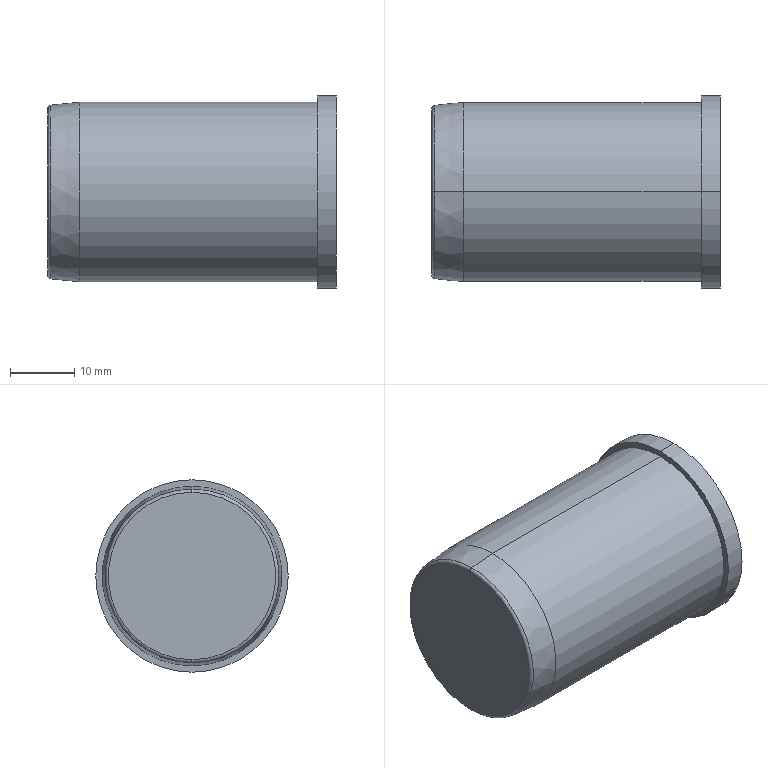Part | STEP file | Handlebar end grip | 1 solid | 14 faces | box 45 x 30 x 30 mm | volume 14675 mm3 | cylinder 6 | plane 4 | torus 2 | cone 2 | commonest cylinder face diameters 20 x2 28 x2 30 x2
STEP:
#1=CARTESIAN_POINT('',(0.,0.,0.));
#2=DIRECTION('',(0.,0.,1.));
#3=DIRECTION('',(1.,0.,0.));
#4=AXIS2_PLACEMENT_3D('',#1,#2,#3);
#5=CARTESIAN_POINT('',(0.,0.,13.048));
#6=VERTEX_POINT('',#5);
#7=CARTESIAN_POINT('',(0.,0.,-13.048));
#8=VERTEX_POINT('',#7);
#9=CARTESIAN_POINT('',(0.,0.,0.));
#10=DIRECTION('',(-1.,0.,0.));
#11=DIRECTION('',(0.,0.,-1.));
#12=AXIS2_PLACEMENT_3D('',#9,#10,#11);
#13=CIRCLE('',#12,13.048);
#14=CARTESIAN_POINT('',(0.5,0.,0.));
#15=DIRECTION('',(1.,0.,0.));
#16=DIRECTION('',(0.,0.,-1.));
#17=AXIS2_PLACEMENT_3D('',#14,#15,#16);
#18=TOROIDAL_SURFACE('',#17,13.048,0.5);
#19=CARTESIAN_POINT('',(6.283,4.712));
#20=DIRECTION('',(-1.,0.));
#21=VECTOR('',#20,1.);
#22=LINE('',#19,#21);
#23=(GEOMETRIC_REPRESENTATION_CONTEXT(2)PARAMETRIC_REPRESENTATION_CONTEXT()REPRESENTATION_CONTEXT('',''));
#24=DEFINITIONAL_REPRESENTATION('',(#22),#23);
#25=PCURVE('',#18,#24);
#26=CARTESIAN_POINT('',(0.,0.,0.));
#27=DIRECTION('',(1.,0.,0.));
#28=DIRECTION('',(0.,0.,-1.));
#29=AXIS2_PLACEMENT_3D('',#26,#27,#28);
#30=PLANE('',#29);
#31=CARTESIAN_POINT('',(13.048,0.));
#32=CARTESIAN_POINT('',(13.048,-22.599));
#33=CARTESIAN_POINT('',(-6.524,-11.299));
#34=CARTESIAN_POINT('',(-26.095,0.));
#35=CARTESIAN_POINT('',(-6.524,11.299));
#36=CARTESIAN_POINT('',(13.048,22.599));
#37=CARTESIAN_POINT('',(13.048,0.));
#38=(BOUNDED_CURVE()B_SPLINE_CURVE(2,(#31,#32,#33,#34,#35,#36,#37),.UNSPECIFIED.,.T.,.F.)B_SPLINE_CURVE_WITH_KNOTS((1,2,2,2,2,1),(-2.094,0.,2.094,4.189,6.283,8.378),.UNSPECIFIED.)CURVE()GEOMETRIC_REPRESENTATION_ITEM()RATIONAL_B_SPLINE_CURVE((1.,0.5,1.,0.5,1.,0.5,1.))REPRESENTATION_ITEM(''));
#39=(GEOMETRIC_REPRESENTATION_CONTEXT(2)PARAMETRIC_REPRESENTATION_CONTEXT()REPRESENTATION_CONTEXT('',''));
#40=DEFINITIONAL_REPRESENTATION('',(#38),#39);
#41=PCURVE('',#30,#40);
#42=SURFACE_CURVE('',#13,(#25,#41),.PCURVE_S1.);
#43=EDGE_CURVE('',#6,#8,#42,.T.);
#44=ORIENTED_EDGE('',*,*,#43,.F.);
#45=CARTESIAN_POINT('',(0.4502,0.,13.545));
#46=VERTEX_POINT('',#45);
#47=CARTESIAN_POINT('',(0.5,0.,13.048));
#48=DIRECTION('',(0.,1.,0.));
#49=DIRECTION('',(0.,0.,1.));
#50=AXIS2_PLACEMENT_3D('',#47,#48,#49);
#51=CIRCLE('',#50,0.5);
#52=CARTESIAN_POINT('',(3.142,0.));
#53=DIRECTION('',(0.,1.));
#54=VECTOR('',#53,1.);
#55=LINE('',#52,#54);
#56=(GEOMETRIC_REPRESENTATION_CONTEXT(2)PARAMETRIC_REPRESENTATION_CONTEXT()REPRESENTATION_CONTEXT('',''));
#57=DEFINITIONAL_REPRESENTATION('',(#55),#56);
#58=PCURVE('',#18,#57);
#59=CARTESIAN_POINT('',(0.5,0.,0.));
#60=DIRECTION('',(1.,0.,0.));
#61=DIRECTION('',(0.,0.,-1.));
#62=AXIS2_PLACEMENT_3D('',#59,#60,#61);
#63=TOROIDAL_SURFACE('',#62,13.048,0.5);
#64=CARTESIAN_POINT('',(3.142,0.));
#65=DIRECTION('',(0.,1.));
#66=VECTOR('',#65,1.);
#67=LINE('',#64,#66);
#68=(GEOMETRIC_REPRESENTATION_CONTEXT(2)PARAMETRIC_REPRESENTATION_CONTEXT()REPRESENTATION_CONTEXT('',''));
#69=DEFINITIONAL_REPRESENTATION('',(#67),#68);
#70=PCURVE('',#63,#69);
#71=SURFACE_CURVE('',#51,(#58,#70),.PCURVE_S1.);
#72=EDGE_CURVE('',#6,#46,#71,.T.);
#73=ORIENTED_EDGE('',*,*,#72,.T.);
#74=CARTESIAN_POINT('',(0.4502,0.,-13.545));
#75=VERTEX_POINT('',#74);
#76=CARTESIAN_POINT('',(0.4502,0.,0.));
#77=DIRECTION('',(1.,0.,0.));
#78=DIRECTION('',(0.,0.,-1.));
#79=AXIS2_PLACEMENT_3D('',#76,#77,#78);
#80=CIRCLE('',#79,13.545);
#81=CARTESIAN_POINT('',(0.,6.184));
#82=DIRECTION('',(1.,0.));
#83=VECTOR('',#82,1.);
#84=LINE('',#81,#83);
#85=(GEOMETRIC_REPRESENTATION_CONTEXT(2)PARAMETRIC_REPRESENTATION_CONTEXT()REPRESENTATION_CONTEXT('',''));
#86=DEFINITIONAL_REPRESENTATION('',(#84),#85);
#87=PCURVE('',#18,#86);
#88=CARTESIAN_POINT('',(0.,0.,0.));
#89=DIRECTION('',(1.,0.,0.));
#90=DIRECTION('',(0.,0.,-1.));
#91=AXIS2_PLACEMENT_3D('',#88,#89,#90);
#92=CONICAL_SURFACE('',#91,13.5,0.09967);
#93=CARTESIAN_POINT('',(0.,0.4502));
#94=DIRECTION('',(1.,0.));
#95=VECTOR('',#94,1.);
#96=LINE('',#93,#95);
#97=(GEOMETRIC_REPRESENTATION_CONTEXT(2)PARAMETRIC_REPRESENTATION_CONTEXT()REPRESENTATION_CONTEXT('',''));
#98=DEFINITIONAL_REPRESENTATION('',(#96),#97);
#99=PCURVE('',#92,#98);
#100=SURFACE_CURVE('',#80,(#87,#99),.PCURVE_S1.);
#101=EDGE_CURVE('',#75,#46,#100,.T.);
#102=ORIENTED_EDGE('',*,*,#101,.F.);
#103=CARTESIAN_POINT('',(0.5,0.,-13.048));
#104=DIRECTION('',(0.,-1.,0.));
#105=DIRECTION('',(0.,0.,-1.));
#106=AXIS2_PLACEMENT_3D('',#103,#104,#105);
#107=CIRCLE('',#106,0.5);
#108=CARTESIAN_POINT('',(0.,0.));
#109=DIRECTION('',(0.,1.));
#110=VECTOR('',#109,1.);
#111=LINE('',#108,#110);
#112=(GEOMETRIC_REPRESENTATION_CONTEXT(2)PARAMETRIC_REPRESENTATION_CONTEXT()REPRESENTATION_CONTEXT('',''));
#113=DEFINITIONAL_REPRESENTATION('',(#111),#112);
#114=PCURVE('',#18,#113);
#115=CARTESIAN_POINT('',(6.283,0.));
#116=DIRECTION('',(0.,1.));
#117=VECTOR('',#116,1.);
#118=LINE('',#115,#117);
#119=(GEOMETRIC_REPRESENTATION_CONTEXT(2)PARAMETRIC_REPRESENTATION_CONTEXT()REPRESENTATION_CONTEXT('',''));
#120=DEFINITIONAL_REPRESENTATION('',(#118),#119);
#121=PCURVE('',#63,#120);
#122=SURFACE_CURVE('',#107,(#114,#121),.PCURVE_S1.);
#123=EDGE_CURVE('',#8,#75,#122,.T.);
#124=ORIENTED_EDGE('',*,*,#123,.F.);
#125=EDGE_LOOP('',(#44,#73,#102,#124));
#126=FACE_BOUND('',#125,.T.);
#127=ADVANCED_FACE('',(#126),#18,.T.);
#128=ORIENTED_EDGE('',*,*,#101,.T.);
#129=CARTESIAN_POINT('',(5.,0.,14.));
#130=VERTEX_POINT('',#129);
#131=CARTESIAN_POINT('',(0.,0.,13.5));
#132=DIRECTION('',(0.995,0.,0.0995));
#133=VECTOR('',#132,1.);
#134=LINE('',#131,#133);
#135=CARTESIAN_POINT('',(3.142,0.));
#136=DIRECTION('',(0.,1.));
#137=VECTOR('',#136,1.);
#138=LINE('',#135,#137);
#139=(GEOMETRIC_REPRESENTATION_CONTEXT(2)PARAMETRIC_REPRESENTATION_CONTEXT()REPRESENTATION_CONTEXT('',''));
#140=DEFINITIONAL_REPRESENTATION('',(#138),#139);
#141=PCURVE('',#92,#140);
#142=CARTESIAN_POINT('',(0.,0.,0.));
#143=DIRECTION('',(1.,0.,0.));
#144=DIRECTION('',(0.,0.,-1.));
#145=AXIS2_PLACEMENT_3D('',#142,#143,#144);
#146=CONICAL_SURFACE('',#145,13.5,0.09967);
#147=CARTESIAN_POINT('',(3.142,0.));
#148=DIRECTION('',(0.,1.));
#149=VECTOR('',#148,1.);
#150=LINE('',#147,#149);
#151=(GEOMETRIC_REPRESENTATION_CONTEXT(2)PARAMETRIC_REPRESENTATION_CONTEXT()REPRESENTATION_CONTEXT('',''));
#152=DEFINITIONAL_REPRESENTATION('',(#150),#151);
#153=PCURVE('',#146,#152);
#154=SURFACE_CURVE('',#134,(#141,#153),.PCURVE_S1.);
#155=EDGE_CURVE('',#46,#130,#154,.T.);
#156=ORIENTED_EDGE('',*,*,#155,.T.);
#157=CARTESIAN_POINT('',(5.,0.,-14.));
#158=VERTEX_POINT('',#157);
#159=CARTESIAN_POINT('',(5.,0.,0.));
#160=DIRECTION('',(1.,0.,0.));
#161=DIRECTION('',(0.,0.,-1.));
#162=AXIS2_PLACEMENT_3D('',#159,#160,#161);
#163=CIRCLE('',#162,14.);
#164=CARTESIAN_POINT('',(0.,5.));
#165=DIRECTION('',(1.,0.));
#166=VECTOR('',#165,1.);
#167=LINE('',#164,#166);
#168=(GEOMETRIC_REPRESENTATION_CONTEXT(2)PARAMETRIC_REPRESENTATION_CONTEXT()REPRESENTATION_CONTEXT('',''));
#169=DEFINITIONAL_REPRESENTATION('',(#167),#168);
#170=PCURVE('',#92,#169);
#171=CARTESIAN_POINT('',(3.,0.,0.));
#172=DIRECTION('',(-1.,0.,0.));
#173=DIRECTION('',(0.,0.,1.));
#174=AXIS2_PLACEMENT_3D('',#171,#172,#173);
#175=CYLINDRICAL_SURFACE('',#174,14.);
#176=CARTESIAN_POINT('',(3.142,-2.));
#177=DIRECTION('',(-1.,0.));
#178=VECTOR('',#177,1.);
#179=LINE('',#176,#178);
#180=(GEOMETRIC_REPRESENTATION_CONTEXT(2)PARAMETRIC_REPRESENTATION_CONTEXT()REPRESENTATION_CONTEXT('',''));
#181=DEFINITIONAL_REPRESENTATION('',(#179),#180);
#182=PCURVE('',#175,#181);
#183=SURFACE_CURVE('',#163,(#170,#182),.PCURVE_S1.);
#184=EDGE_CURVE('',#158,#130,#183,.T.);
#185=ORIENTED_EDGE('',*,*,#184,.F.);
#186=CARTESIAN_POINT('',(0.,0.,-13.5));
#187=DIRECTION('',(0.995,0.,-0.0995));
#188=VECTOR('',#187,1.);
#189=LINE('',#186,#188);
#190=CARTESIAN_POINT('',(0.,0.));
#191=DIRECTION('',(0.,1.));
#192=VECTOR('',#191,1.);
#193=LINE('',#190,#192);
#194=(GEOMETRIC_REPRESENTATION_CONTEXT(2)PARAMETRIC_REPRESENTATION_CONTEXT()REPRESENTATION_CONTEXT('',''));
#195=DEFINITIONAL_REPRESENTATION('',(#193),#194);
#196=PCURVE('',#92,#195);
#197=CARTESIAN_POINT('',(6.283,0.));
#198=DIRECTION('',(0.,1.));
#199=VECTOR('',#198,1.);
#200=LINE('',#197,#199);
#201=(GEOMETRIC_REPRESENTATION_CONTEXT(2)PARAMETRIC_REPRESENTATION_CONTEXT()REPRESENTATION_CONTEXT('',''));
#202=DEFINITIONAL_REPRESENTATION('',(#200),#201);
#203=PCURVE('',#146,#202);
#204=SURFACE_CURVE('',#189,(#196,#203),.PCURVE_S1.);
#205=EDGE_CURVE('',#75,#158,#204,.T.);
#206=ORIENTED_EDGE('',*,*,#205,.F.);
#207=EDGE_LOOP('',(#128,#156,#185,#206));
#208=FACE_BOUND('',#207,.T.);
#209=ADVANCED_FACE('',(#208),#92,.T.);
#210=CARTESIAN_POINT('',(45.,0.,10.));
#211=VERTEX_POINT('',#210);
#212=CARTESIAN_POINT('',(3.,0.,10.));
#213=VERTEX_POINT('',#212);
#214=CARTESIAN_POINT('',(3.,0.,10.));
#215=DIRECTION('',(-1.,0.,0.));
#216=VECTOR('',#215,1.);
#217=LINE('',#214,#216);
#218=CARTESIAN_POINT('',(3.,0.,0.));
#219=DIRECTION('',(-1.,0.,0.));
#220=DIRECTION('',(0.,0.,1.));
#221=AXIS2_PLACEMENT_3D('',#218,#219,#220);
#222=CYLINDRICAL_SURFACE('',#221,10.);
#223=CARTESIAN_POINT('',(6.283,0.));
#224=DIRECTION('',(0.,1.));
#225=VECTOR('',#224,1.);
#226=LINE('',#223,#225);
#227=(GEOMETRIC_REPRESENTATION_CONTEXT(2)PARAMETRIC_REPRESENTATION_CONTEXT()REPRESENTATION_CONTEXT('',''));
#228=DEFINITIONAL_REPRESENTATION('',(#226),#227);
#229=PCURVE('',#222,#228);
#230=CARTESIAN_POINT('',(3.,0.,0.));
#231=DIRECTION('',(-1.,0.,0.));
#232=DIRECTION('',(0.,0.,1.));
#233=AXIS2_PLACEMENT_3D('',#230,#231,#232);
#234=CYLINDRICAL_SURFACE('',#233,10.);
#235=CARTESIAN_POINT('',(0.,0.));
#236=DIRECTION('',(0.,1.));
#237=VECTOR('',#236,1.);
#238=LINE('',#235,#237);
#239=(GEOMETRIC_REPRESENTATION_CONTEXT(2)PARAMETRIC_REPRESENTATION_CONTEXT()REPRESENTATION_CONTEXT('',''));
#240=DEFINITIONAL_REPRESENTATION('',(#238),#239);
#241=PCURVE('',#234,#240);
#242=SURFACE_CURVE('',#217,(#229,#241),.PCURVE_S1.);
#243=EDGE_CURVE('',#211,#213,#242,.T.);
#244=ORIENTED_EDGE('',*,*,#243,.T.);
#245=CARTESIAN_POINT('',(3.,0.,-10.));
#246=VERTEX_POINT('',#245);
#247=CARTESIAN_POINT('',(3.,0.,0.));
#248=DIRECTION('',(-1.,0.,0.));
#249=DIRECTION('',(0.,0.,1.));
#250=AXIS2_PLACEMENT_3D('',#247,#248,#249);
#251=CIRCLE('',#250,10.);
#252=CARTESIAN_POINT('',(0.,0.));
#253=DIRECTION('',(1.,0.));
#254=VECTOR('',#253,1.);
#255=LINE('',#252,#254);
#256=(GEOMETRIC_REPRESENTATION_CONTEXT(2)PARAMETRIC_REPRESENTATION_CONTEXT()REPRESENTATION_CONTEXT('',''));
#257=DEFINITIONAL_REPRESENTATION('',(#255),#256);
#258=PCURVE('',#222,#257);
#259=CARTESIAN_POINT('',(3.,0.,-10.));
#260=DIRECTION('',(-1.,0.,0.));
#261=DIRECTION('',(0.,0.,1.));
#262=AXIS2_PLACEMENT_3D('',#259,#260,#261);
#263=PLANE('',#262);
#264=CARTESIAN_POINT('',(10.,0.));
#265=DIRECTION('',(1.,0.));
#266=AXIS2_PLACEMENT_2D('',#264,#265);
#267=CIRCLE('',#266,10.);
#268=(GEOMETRIC_REPRESENTATION_CONTEXT(2)PARAMETRIC_REPRESENTATION_CONTEXT()REPRESENTATION_CONTEXT('',''));
#269=DEFINITIONAL_REPRESENTATION('',(#267),#268);
#270=PCURVE('',#263,#269);
#271=SURFACE_CURVE('',#251,(#258,#270),.PCURVE_S1.);
#272=EDGE_CURVE('',#246,#213,#271,.T.);
#273=ORIENTED_EDGE('',*,*,#272,.F.);
#274=CARTESIAN_POINT('',(45.,0.,-10.));
#275=VERTEX_POINT('',#274);
#276=CARTESIAN_POINT('',(3.,0.,-10.));
#277=DIRECTION('',(-1.,0.,0.));
#278=VECTOR('',#277,1.);
#279=LINE('',#276,#278);
#280=CARTESIAN_POINT('',(3.142,0.));
#281=DIRECTION('',(0.,1.));
#282=VECTOR('',#281,1.);
#283=LINE('',#280,#282);
#284=(GEOMETRIC_REPRESENTATION_CONTEXT(2)PARAMETRIC_REPRESENTATION_CONTEXT()REPRESENTATION_CONTEXT('',''));
#285=DEFINITIONAL_REPRESENTATION('',(#283),#284);
#286=PCURVE('',#222,#285);
#287=CARTESIAN_POINT('',(3.142,0.));
#288=DIRECTION('',(0.,1.));
#289=VECTOR('',#288,1.);
#290=LINE('',#287,#289);
#291=(GEOMETRIC_REPRESENTATION_CONTEXT(2)PARAMETRIC_REPRESENTATION_CONTEXT()REPRESENTATION_CONTEXT('',''));
#292=DEFINITIONAL_REPRESENTATION('',(#290),#291);
#293=PCURVE('',#234,#292);
#294=SURFACE_CURVE('',#279,(#286,#293),.PCURVE_S1.);
#295=EDGE_CURVE('',#275,#246,#294,.T.);
#296=ORIENTED_EDGE('',*,*,#295,.F.);
#297=CARTESIAN_POINT('',(45.,0.,0.));
#298=DIRECTION('',(-1.,0.,0.));
#299=DIRECTION('',(0.,0.,1.));
#300=AXIS2_PLACEMENT_3D('',#297,#298,#299);
#301=CIRCLE('',#300,10.);
#302=CARTESIAN_POINT('',(0.,-42.));
#303=DIRECTION('',(1.,0.));
#304=VECTOR('',#303,1.);
#305=LINE('',#302,#304);
#306=(GEOMETRIC_REPRESENTATION_CONTEXT(2)PARAMETRIC_REPRESENTATION_CONTEXT()REPRESENTATION_CONTEXT('',''));
#307=DEFINITIONAL_REPRESENTATION('',(#305),#306);
#308=PCURVE('',#222,#307);
#309=CARTESIAN_POINT('',(45.,0.,-10.));
#310=DIRECTION('',(-1.,0.,0.));
#311=DIRECTION('',(0.,0.,1.));
#312=AXIS2_PLACEMENT_3D('',#309,#310,#311);
#313=PLANE('',#312);
#314=CARTESIAN_POINT('',(10.,0.));
#315=DIRECTION('',(1.,0.));
#316=AXIS2_PLACEMENT_2D('',#314,#315);
#317=CIRCLE('',#316,10.);
#318=(GEOMETRIC_REPRESENTATION_CONTEXT(2)PARAMETRIC_REPRESENTATION_CONTEXT()REPRESENTATION_CONTEXT('',''));
#319=DEFINITIONAL_REPRESENTATION('',(#317),#318);
#320=PCURVE('',#313,#319);
#321=SURFACE_CURVE('',#301,(#308,#320),.PCURVE_S1.);
#322=EDGE_CURVE('',#275,#211,#321,.T.);
#323=ORIENTED_EDGE('',*,*,#322,.T.);
#324=EDGE_LOOP('',(#244,#273,#296,#323));
#325=FACE_BOUND('',#324,.F.);
#326=ADVANCED_FACE('',(#325),#222,.F.);
#327=CARTESIAN_POINT('',(45.,0.,15.));
#328=VERTEX_POINT('',#327);
#329=CARTESIAN_POINT('',(45.,0.,-15.));
#330=VERTEX_POINT('',#329);
#331=CARTESIAN_POINT('',(45.,0.,0.));
#332=DIRECTION('',(-1.,0.,0.));
#333=DIRECTION('',(0.,0.,1.));
#334=AXIS2_PLACEMENT_3D('',#331,#332,#333);
#335=CIRCLE('',#334,15.);
#336=CARTESIAN_POINT('',(3.,0.,0.));
#337=DIRECTION('',(-1.,0.,0.));
#338=DIRECTION('',(0.,0.,1.));
#339=AXIS2_PLACEMENT_3D('',#336,#337,#338);
#340=CYLINDRICAL_SURFACE('',#339,15.);
#341=CARTESIAN_POINT('',(0.,-42.));
#342=DIRECTION('',(1.,0.));
#343=VECTOR('',#342,1.);
#344=LINE('',#341,#343);
#345=(GEOMETRIC_REPRESENTATION_CONTEXT(2)PARAMETRIC_REPRESENTATION_CONTEXT()REPRESENTATION_CONTEXT('',''));
#346=DEFINITIONAL_REPRESENTATION('',(#344),#345);
#347=PCURVE('',#340,#346);
#348=CARTESIAN_POINT('',(10.,0.));
#349=DIRECTION('',(1.,0.));
#350=AXIS2_PLACEMENT_2D('',#348,#349);
#351=CIRCLE('',#350,15.);
#352=(GEOMETRIC_REPRESENTATION_CONTEXT(2)PARAMETRIC_REPRESENTATION_CONTEXT()REPRESENTATION_CONTEXT('',''));
#353=DEFINITIONAL_REPRESENTATION('',(#351),#352);
#354=PCURVE('',#313,#353);
#355=SURFACE_CURVE('',#335,(#347,#354),.PCURVE_S1.);
#356=EDGE_CURVE('',#328,#330,#355,.T.);
#357=ORIENTED_EDGE('',*,*,#356,.T.);
#358=CARTESIAN_POINT('',(42.,0.,-15.));
#359=VERTEX_POINT('',#358);
#360=CARTESIAN_POINT('',(3.,0.,-15.));
#361=DIRECTION('',(-1.,0.,0.));
#362=VECTOR('',#361,1.);
#363=LINE('',#360,#362);
#364=CARTESIAN_POINT('',(3.142,0.));
#365=DIRECTION('',(0.,1.));
#366=VECTOR('',#365,1.);
#367=LINE('',#364,#366);
#368=(GEOMETRIC_REPRESENTATION_CONTEXT(2)PARAMETRIC_REPRESENTATION_CONTEXT()REPRESENTATION_CONTEXT('',''));
#369=DEFINITIONAL_REPRESENTATION('',(#367),#368);
#370=PCURVE('',#340,#369);
#371=CARTESIAN_POINT('',(3.,0.,0.));
#372=DIRECTION('',(-1.,0.,0.));
#373=DIRECTION('',(0.,0.,1.));
#374=AXIS2_PLACEMENT_3D('',#371,#372,#373);
#375=CYLINDRICAL_SURFACE('',#374,15.);
#376=CARTESIAN_POINT('',(3.142,0.));
#377=DIRECTION('',(0.,1.));
#378=VECTOR('',#377,1.);
#379=LINE('',#376,#378);
#380=(GEOMETRIC_REPRESENTATION_CONTEXT(2)PARAMETRIC_REPRESENTATION_CONTEXT()REPRESENTATION_CONTEXT('',''));
#381=DEFINITIONAL_REPRESENTATION('',(#379),#380);
#382=PCURVE('',#375,#381);
#383=SURFACE_CURVE('',#363,(#370,#382),.PCURVE_S1.);
#384=EDGE_CURVE('',#330,#359,#383,.T.);
#385=ORIENTED_EDGE('',*,*,#384,.T.);
#386=CARTESIAN_POINT('',(42.,0.,15.));
#387=VERTEX_POINT('',#386);
#388=CARTESIAN_POINT('',(42.,0.,0.));
#389=DIRECTION('',(-1.,0.,0.));
#390=DIRECTION('',(0.,0.,1.));
#391=AXIS2_PLACEMENT_3D('',#388,#389,#390);
#392=CIRCLE('',#391,15.);
#393=CARTESIAN_POINT('',(0.,-39.));
#394=DIRECTION('',(1.,0.));
#395=VECTOR('',#394,1.);
#396=LINE('',#393,#395);
#397=(GEOMETRIC_REPRESENTATION_CONTEXT(2)PARAMETRIC_REPRESENTATION_CONTEXT()REPRESENTATION_CONTEXT('',''));
#398=DEFINITIONAL_REPRESENTATION('',(#396),#397);
#399=PCURVE('',#340,#398);
#400=CARTESIAN_POINT('',(42.,0.,-14.));
#401=DIRECTION('',(1.,0.,0.));
#402=DIRECTION('',(0.,0.,-1.));
#403=AXIS2_PLACEMENT_3D('',#400,#401,#402);
#404=PLANE('',#403);
#405=CARTESIAN_POINT('',(-29.,0.));
#406=CARTESIAN_POINT('',(-29.,25.981));
#407=CARTESIAN_POINT('',(-6.5,12.99));
#408=CARTESIAN_POINT('',(16.,0.));
#409=CARTESIAN_POINT('',(-6.5,-12.99));
#410=CARTESIAN_POINT('',(-29.,-25.981));
#411=CARTESIAN_POINT('',(-29.,0.));
#412=(BOUNDED_CURVE()B_SPLINE_CURVE(2,(#405,#406,#407,#408,#409,#410,#411),.UNSPECIFIED.,.T.,.F.)B_SPLINE_CURVE_WITH_KNOTS((1,2,2,2,2,1),(-2.094,0.,2.094,4.189,6.283,8.378),.UNSPECIFIED.)CURVE()GEOMETRIC_REPRESENTATION_ITEM()RATIONAL_B_SPLINE_CURVE((1.,0.5,1.,0.5,1.,0.5,1.))REPRESENTATION_ITEM(''));
#413=(GEOMETRIC_REPRESENTATION_CONTEXT(2)PARAMETRIC_REPRESENTATION_CONTEXT()REPRESENTATION_CONTEXT('',''));
#414=DEFINITIONAL_REPRESENTATION('',(#412),#413);
#415=PCURVE('',#404,#414);
#416=SURFACE_CURVE('',#392,(#399,#415),.PCURVE_S1.);
#417=EDGE_CURVE('',#387,#359,#416,.T.);
#418=ORIENTED_EDGE('',*,*,#417,.F.);
#419=CARTESIAN_POINT('',(3.,0.,15.));
#420=DIRECTION('',(-1.,0.,0.));
#421=VECTOR('',#420,1.);
#422=LINE('',#419,#421);
#423=CARTESIAN_POINT('',(0.,0.));
#424=DIRECTION('',(0.,1.));
#425=VECTOR('',#424,1.);
#426=LINE('',#423,#425);
#427=(GEOMETRIC_REPRESENTATION_CONTEXT(2)PARAMETRIC_REPRESENTATION_CONTEXT()REPRESENTATION_CONTEXT('',''));
#428=DEFINITIONAL_REPRESENTATION('',(#426),#427);
#429=PCURVE('',#340,#428);
#430=CARTESIAN_POINT('',(6.283,0.));
#431=DIRECTION('',(0.,1.));
#432=VECTOR('',#431,1.);
#433=LINE('',#430,#432);
#434=(GEOMETRIC_REPRESENTATION_CONTEXT(2)PARAMETRIC_REPRESENTATION_CONTEXT()REPRESENTATION_CONTEXT('',''));
#435=DEFINITIONAL_REPRESENTATION('',(#433),#434);
#436=PCURVE('',#375,#435);
#437=SURFACE_CURVE('',#422,(#429,#436),.PCURVE_S1.);
#438=EDGE_CURVE('',#328,#387,#437,.T.);
#439=ORIENTED_EDGE('',*,*,#438,.F.);
#440=EDGE_LOOP('',(#357,#385,#418,#439));
#441=FACE_BOUND('',#440,.T.);
#442=ADVANCED_FACE('',(#441),#340,.T.);
#443=CARTESIAN_POINT('',(42.,0.,14.));
#444=VERTEX_POINT('',#443);
#445=CARTESIAN_POINT('',(42.,0.,-14.));
#446=VERTEX_POINT('',#445);
#447=CARTESIAN_POINT('',(42.,0.,0.));
#448=DIRECTION('',(-1.,0.,0.));
#449=DIRECTION('',(0.,0.,1.));
#450=AXIS2_PLACEMENT_3D('',#447,#448,#449);
#451=CIRCLE('',#450,14.);
#452=CARTESIAN_POINT('',(0.,-39.));
#453=DIRECTION('',(1.,0.));
#454=VECTOR('',#453,1.);
#455=LINE('',#452,#454);
#456=(GEOMETRIC_REPRESENTATION_CONTEXT(2)PARAMETRIC_REPRESENTATION_CONTEXT()REPRESENTATION_CONTEXT('',''));
#457=DEFINITIONAL_REPRESENTATION('',(#455),#456);
#458=PCURVE('',#175,#457);
#459=CARTESIAN_POINT('',(-28.,0.));
#460=CARTESIAN_POINT('',(-28.,24.249));
#461=CARTESIAN_POINT('',(-7.,12.124));
#462=CARTESIAN_POINT('',(14.,0.));
#463=CARTESIAN_POINT('',(-7.,-12.124));
#464=CARTESIAN_POINT('',(-28.,-24.249));
#465=CARTESIAN_POINT('',(-28.,0.));
#466=(BOUNDED_CURVE()B_SPLINE_CURVE(2,(#459,#460,#461,#462,#463,#464,#465),.UNSPECIFIED.,.T.,.F.)B_SPLINE_CURVE_WITH_KNOTS((1,2,2,2,2,1),(-2.094,0.,2.094,4.189,6.283,8.378),.UNSPECIFIED.)CURVE()GEOMETRIC_REPRESENTATION_ITEM()RATIONAL_B_SPLINE_CURVE((1.,0.5,1.,0.5,1.,0.5,1.))REPRESENTATION_ITEM(''));
#467=(GEOMETRIC_REPRESENTATION_CONTEXT(2)PARAMETRIC_REPRESENTATION_CONTEXT()REPRESENTATION_CONTEXT('',''));
#468=DEFINITIONAL_REPRESENTATION('',(#466),#467);
#469=PCURVE('',#404,#468);
#470=SURFACE_CURVE('',#451,(#458,#469),.PCURVE_S1.);
#471=EDGE_CURVE('',#444,#446,#470,.T.);
#472=ORIENTED_EDGE('',*,*,#471,.T.);
#473=CARTESIAN_POINT('',(3.,0.,-14.));
#474=DIRECTION('',(-1.,0.,0.));
#475=VECTOR('',#474,1.);
#476=LINE('',#473,#475);
#477=CARTESIAN_POINT('',(3.142,0.));
#478=DIRECTION('',(0.,1.));
#479=VECTOR('',#478,1.);
#480=LINE('',#477,#479);
#481=(GEOMETRIC_REPRESENTATION_CONTEXT(2)PARAMETRIC_REPRESENTATION_CONTEXT()REPRESENTATION_CONTEXT('',''));
#482=DEFINITIONAL_REPRESENTATION('',(#480),#481);
#483=PCURVE('',#175,#482);
#484=CARTESIAN_POINT('',(3.,0.,0.));
#485=DIRECTION('',(-1.,0.,0.));
#486=DIRECTION('',(0.,0.,1.));
#487=AXIS2_PLACEMENT_3D('',#484,#485,#486);
#488=CYLINDRICAL_SURFACE('',#487,14.);
#489=CARTESIAN_POINT('',(3.142,0.));
#490=DIRECTION('',(0.,1.));
#491=VECTOR('',#490,1.);
#492=LINE('',#489,#491);
#493=(GEOMETRIC_REPRESENTATION_CONTEXT(2)PARAMETRIC_REPRESENTATION_CONTEXT()REPRESENTATION_CONTEXT('',''));
#494=DEFINITIONAL_REPRESENTATION('',(#492),#493);
#495=PCURVE('',#488,#494);
#496=SURFACE_CURVE('',#476,(#483,#495),.PCURVE_S1.);
#497=EDGE_CURVE('',#446,#158,#496,.T.);
#498=ORIENTED_EDGE('',*,*,#497,.T.);
#499=ORIENTED_EDGE('',*,*,#184,.T.);
#500=CARTESIAN_POINT('',(3.,0.,14.));
#501=DIRECTION('',(-1.,0.,0.));
#502=VECTOR('',#501,1.);
#503=LINE('',#500,#502);
#504=CARTESIAN_POINT('',(0.,0.));
#505=DIRECTION('',(0.,1.));
#506=VECTOR('',#505,1.);
#507=LINE('',#504,#506);
#508=(GEOMETRIC_REPRESENTATION_CONTEXT(2)PARAMETRIC_REPRESENTATION_CONTEXT()REPRESENTATION_CONTEXT('',''));
#509=DEFINITIONAL_REPRESENTATION('',(#507),#508);
#510=PCURVE('',#175,#509);
#511=CARTESIAN_POINT('',(6.283,0.));
#512=DIRECTION('',(0.,1.));
#513=VECTOR('',#512,1.);
#514=LINE('',#511,#513);
#515=(GEOMETRIC_REPRESENTATION_CONTEXT(2)PARAMETRIC_REPRESENTATION_CONTEXT()REPRESENTATION_CONTEXT('',''));
#516=DEFINITIONAL_REPRESENTATION('',(#514),#515);
#517=PCURVE('',#488,#516);
#518=SURFACE_CURVE('',#503,(#510,#517),.PCURVE_S1.);
#519=EDGE_CURVE('',#444,#130,#518,.T.);
#520=ORIENTED_EDGE('',*,*,#519,.F.);
#521=EDGE_LOOP('',(#472,#498,#499,#520));
#522=FACE_BOUND('',#521,.T.);
#523=ADVANCED_FACE('',(#522),#175,.T.);
#524=CARTESIAN_POINT('',(0.,0.,0.));
#525=DIRECTION('',(-1.,0.,0.));
#526=DIRECTION('',(0.,0.,-1.));
#527=AXIS2_PLACEMENT_3D('',#524,#525,#526);
#528=CIRCLE('',#527,13.048);
#529=CARTESIAN_POINT('',(13.048,0.));
#530=CARTESIAN_POINT('',(13.048,-22.599));
#531=CARTESIAN_POINT('',(-6.524,-11.299));
#532=CARTESIAN_POINT('',(-26.095,0.));
#533=CARTESIAN_POINT('',(-6.524,11.299));
#534=CARTESIAN_POINT('',(13.048,22.599));
#535=CARTESIAN_POINT('',(13.048,0.));
#536=(BOUNDED_CURVE()B_SPLINE_CURVE(2,(#529,#530,#531,#532,#533,#534,#535),.UNSPECIFIED.,.T.,.F.)B_SPLINE_CURVE_WITH_KNOTS((1,2,2,2,2,1),(-2.094,0.,2.094,4.189,6.283,8.378),.UNSPECIFIED.)CURVE()GEOMETRIC_REPRESENTATION_ITEM()RATIONAL_B_SPLINE_CURVE((1.,0.5,1.,0.5,1.,0.5,1.))REPRESENTATION_ITEM(''));
#537=(GEOMETRIC_REPRESENTATION_CONTEXT(2)PARAMETRIC_REPRESENTATION_CONTEXT()REPRESENTATION_CONTEXT('',''));
#538=DEFINITIONAL_REPRESENTATION('',(#536),#537);
#539=PCURVE('',#30,#538);
#540=CARTESIAN_POINT('',(6.283,4.712));
#541=DIRECTION('',(-1.,0.));
#542=VECTOR('',#541,1.);
#543=LINE('',#540,#542);
#544=(GEOMETRIC_REPRESENTATION_CONTEXT(2)PARAMETRIC_REPRESENTATION_CONTEXT()REPRESENTATION_CONTEXT('',''));
#545=DEFINITIONAL_REPRESENTATION('',(#543),#544);
#546=PCURVE('',#63,#545);
#547=SURFACE_CURVE('',#528,(#539,#546),.PCURVE_S1.);
#548=EDGE_CURVE('',#8,#6,#547,.T.);
#549=ORIENTED_EDGE('',*,*,#548,.T.);
#550=ORIENTED_EDGE('',*,*,#43,.T.);
#551=EDGE_LOOP('',(#549,#550));
#552=FACE_BOUND('',#551,.T.);
#553=ADVANCED_FACE('',(#552),#30,.F.);
#554=ORIENTED_EDGE('',*,*,#497,.F.);
#555=CARTESIAN_POINT('',(42.,0.,0.));
#556=DIRECTION('',(-1.,0.,0.));
#557=DIRECTION('',(0.,0.,1.));
#558=AXIS2_PLACEMENT_3D('',#555,#556,#557);
#559=CIRCLE('',#558,14.);
#560=CARTESIAN_POINT('',(0.,-39.));
#561=DIRECTION('',(1.,0.));
#562=VECTOR('',#561,1.);
#563=LINE('',#560,#562);
#564=(GEOMETRIC_REPRESENTATION_CONTEXT(2)PARAMETRIC_REPRESENTATION_CONTEXT()REPRESENTATION_CONTEXT('',''));
#565=DEFINITIONAL_REPRESENTATION('',(#563),#564);
#566=PCURVE('',#488,#565);
#567=CARTESIAN_POINT('',(-28.,0.));
#568=CARTESIAN_POINT('',(-28.,24.249));
#569=CARTESIAN_POINT('',(-7.,12.124));
#570=CARTESIAN_POINT('',(14.,0.));
#571=CARTESIAN_POINT('',(-7.,-12.124));
#572=CARTESIAN_POINT('',(-28.,-24.249));
#573=CARTESIAN_POINT('',(-28.,0.));
#574=(BOUNDED_CURVE()B_SPLINE_CURVE(2,(#567,#568,#569,#570,#571,#572,#573),.UNSPECIFIED.,.T.,.F.)B_SPLINE_CURVE_WITH_KNOTS((1,2,2,2,2,1),(-2.094,0.,2.094,4.189,6.283,8.378),.UNSPECIFIED.)CURVE()GEOMETRIC_REPRESENTATION_ITEM()RATIONAL_B_SPLINE_CURVE((1.,0.5,1.,0.5,1.,0.5,1.))REPRESENTATION_ITEM(''));
#575=(GEOMETRIC_REPRESENTATION_CONTEXT(2)PARAMETRIC_REPRESENTATION_CONTEXT()REPRESENTATION_CONTEXT('',''));
#576=DEFINITIONAL_REPRESENTATION('',(#574),#575);
#577=PCURVE('',#404,#576);
#578=SURFACE_CURVE('',#559,(#566,#577),.PCURVE_S1.);
#579=EDGE_CURVE('',#446,#444,#578,.T.);
#580=ORIENTED_EDGE('',*,*,#579,.T.);
#581=ORIENTED_EDGE('',*,*,#519,.T.);
#582=CARTESIAN_POINT('',(5.,0.,0.));
#583=DIRECTION('',(1.,0.,0.));
#584=DIRECTION('',(0.,0.,-1.));
#585=AXIS2_PLACEMENT_3D('',#582,#583,#584);
#586=CIRCLE('',#585,14.);
#587=CARTESIAN_POINT('',(9.425,-2.));
#588=DIRECTION('',(-1.,0.));
#589=VECTOR('',#588,1.);
#590=LINE('',#587,#589);
#591=(GEOMETRIC_REPRESENTATION_CONTEXT(2)PARAMETRIC_REPRESENTATION_CONTEXT()REPRESENTATION_CONTEXT('',''));
#592=DEFINITIONAL_REPRESENTATION('',(#590),#591);
#593=PCURVE('',#488,#592);
#594=CARTESIAN_POINT('',(0.,5.));
#595=DIRECTION('',(1.,0.));
#596=VECTOR('',#595,1.);
#597=LINE('',#594,#596);
#598=(GEOMETRIC_REPRESENTATION_CONTEXT(2)PARAMETRIC_REPRESENTATION_CONTEXT()REPRESENTATION_CONTEXT('',''));
#599=DEFINITIONAL_REPRESENTATION('',(#597),#598);
#600=PCURVE('',#146,#599);
#601=SURFACE_CURVE('',#586,(#593,#600),.PCURVE_S1.);
#602=EDGE_CURVE('',#130,#158,#601,.T.);
#603=ORIENTED_EDGE('',*,*,#602,.T.);
#604=EDGE_LOOP('',(#554,#580,#581,#603));
#605=FACE_BOUND('',#604,.T.);
#606=ADVANCED_FACE('',(#605),#488,.T.);
#607=ORIENTED_EDGE('',*,*,#471,.F.);
#608=ORIENTED_EDGE('',*,*,#579,.F.);
#609=EDGE_LOOP('',(#607,#608));
#610=FACE_BOUND('',#609,.T.);
#611=ORIENTED_EDGE('',*,*,#417,.T.);
#612=CARTESIAN_POINT('',(42.,0.,0.));
#613=DIRECTION('',(-1.,0.,0.));
#614=DIRECTION('',(0.,0.,1.));
#615=AXIS2_PLACEMENT_3D('',#612,#613,#614);
#616=CIRCLE('',#615,15.);
#617=CARTESIAN_POINT('',(-29.,0.));
#618=CARTESIAN_POINT('',(-29.,25.981));
#619=CARTESIAN_POINT('',(-6.5,12.99));
#620=CARTESIAN_POINT('',(16.,0.));
#621=CARTESIAN_POINT('',(-6.5,-12.99));
#622=CARTESIAN_POINT('',(-29.,-25.981));
#623=CARTESIAN_POINT('',(-29.,0.));
#624=(BOUNDED_CURVE()B_SPLINE_CURVE(2,(#617,#618,#619,#620,#621,#622,#623),.UNSPECIFIED.,.T.,.F.)B_SPLINE_CURVE_WITH_KNOTS((1,2,2,2,2,1),(-2.094,0.,2.094,4.189,6.283,8.378),.UNSPECIFIED.)CURVE()GEOMETRIC_REPRESENTATION_ITEM()RATIONAL_B_SPLINE_CURVE((1.,0.5,1.,0.5,1.,0.5,1.))REPRESENTATION_ITEM(''));
#625=(GEOMETRIC_REPRESENTATION_CONTEXT(2)PARAMETRIC_REPRESENTATION_CONTEXT()REPRESENTATION_CONTEXT('',''));
#626=DEFINITIONAL_REPRESENTATION('',(#624),#625);
#627=PCURVE('',#404,#626);
#628=CARTESIAN_POINT('',(0.,-39.));
#629=DIRECTION('',(1.,0.));
#630=VECTOR('',#629,1.);
#631=LINE('',#628,#630);
#632=(GEOMETRIC_REPRESENTATION_CONTEXT(2)PARAMETRIC_REPRESENTATION_CONTEXT()REPRESENTATION_CONTEXT('',''));
#633=DEFINITIONAL_REPRESENTATION('',(#631),#632);
#634=PCURVE('',#375,#633);
#635=SURFACE_CURVE('',#616,(#627,#634),.PCURVE_S1.);
#636=EDGE_CURVE('',#359,#387,#635,.T.);
#637=ORIENTED_EDGE('',*,*,#636,.T.);
#638=EDGE_LOOP('',(#611,#637));
#639=FACE_BOUND('',#638,.T.);
#640=ADVANCED_FACE('',(#610,#639),#404,.F.);
#641=ORIENTED_EDGE('',*,*,#384,.F.);
#642=CARTESIAN_POINT('',(45.,0.,0.));
#643=DIRECTION('',(-1.,0.,0.));
#644=DIRECTION('',(0.,0.,1.));
#645=AXIS2_PLACEMENT_3D('',#642,#643,#644);
#646=CIRCLE('',#645,15.);
#647=CARTESIAN_POINT('',(0.,-42.));
#648=DIRECTION('',(1.,0.));
#649=VECTOR('',#648,1.);
#650=LINE('',#647,#649);
#651=(GEOMETRIC_REPRESENTATION_CONTEXT(2)PARAMETRIC_REPRESENTATION_CONTEXT()REPRESENTATION_CONTEXT('',''));
#652=DEFINITIONAL_REPRESENTATION('',(#650),#651);
#653=PCURVE('',#375,#652);
#654=CARTESIAN_POINT('',(10.,0.));
#655=DIRECTION('',(1.,0.));
#656=AXIS2_PLACEMENT_2D('',#654,#655);
#657=CIRCLE('',#656,15.);
#658=(GEOMETRIC_REPRESENTATION_CONTEXT(2)PARAMETRIC_REPRESENTATION_CONTEXT()REPRESENTATION_CONTEXT('',''));
#659=DEFINITIONAL_REPRESENTATION('',(#657),#658);
#660=PCURVE('',#313,#659);
#661=SURFACE_CURVE('',#646,(#653,#660),.PCURVE_S1.);
#662=EDGE_CURVE('',#330,#328,#661,.T.);
#663=ORIENTED_EDGE('',*,*,#662,.T.);
#664=ORIENTED_EDGE('',*,*,#438,.T.);
#665=ORIENTED_EDGE('',*,*,#636,.F.);
#666=EDGE_LOOP('',(#641,#663,#664,#665));
#667=FACE_BOUND('',#666,.T.);
#668=ADVANCED_FACE('',(#667),#375,.T.);
#669=ORIENTED_EDGE('',*,*,#356,.F.);
#670=ORIENTED_EDGE('',*,*,#662,.F.);
#671=EDGE_LOOP('',(#669,#670));
#672=FACE_BOUND('',#671,.T.);
#673=CARTESIAN_POINT('',(45.,0.,0.));
#674=DIRECTION('',(-1.,0.,0.));
#675=DIRECTION('',(0.,0.,1.));
#676=AXIS2_PLACEMENT_3D('',#673,#674,#675);
#677=CIRCLE('',#676,10.);
#678=CARTESIAN_POINT('',(10.,0.));
#679=DIRECTION('',(1.,0.));
#680=AXIS2_PLACEMENT_2D('',#678,#679);
#681=CIRCLE('',#680,10.);
#682=(GEOMETRIC_REPRESENTATION_CONTEXT(2)PARAMETRIC_REPRESENTATION_CONTEXT()REPRESENTATION_CONTEXT('',''));
#683=DEFINITIONAL_REPRESENTATION('',(#681),#682);
#684=PCURVE('',#313,#683);
#685=CARTESIAN_POINT('',(0.,-42.));
#686=DIRECTION('',(1.,0.));
#687=VECTOR('',#686,1.);
#688=LINE('',#685,#687);
#689=(GEOMETRIC_REPRESENTATION_CONTEXT(2)PARAMETRIC_REPRESENTATION_CONTEXT()REPRESENTATION_CONTEXT('',''));
#690=DEFINITIONAL_REPRESENTATION('',(#688),#689);
#691=PCURVE('',#234,#690);
#692=SURFACE_CURVE('',#677,(#684,#691),.PCURVE_S1.);
#693=EDGE_CURVE('',#211,#275,#692,.T.);
#694=ORIENTED_EDGE('',*,*,#693,.T.);
#695=ORIENTED_EDGE('',*,*,#322,.T.);
#696=EDGE_LOOP('',(#694,#695));
#697=FACE_BOUND('',#696,.T.);
#698=ADVANCED_FACE('',(#672,#697),#313,.F.);
#699=CARTESIAN_POINT('',(3.,0.,0.));
#700=DIRECTION('',(-1.,0.,0.));
#701=DIRECTION('',(0.,0.,1.));
#702=AXIS2_PLACEMENT_3D('',#699,#700,#701);
#703=CIRCLE('',#702,10.);
#704=CARTESIAN_POINT('',(0.,0.));
#705=DIRECTION('',(1.,0.));
#706=VECTOR('',#705,1.);
#707=LINE('',#704,#706);
#708=(GEOMETRIC_REPRESENTATION_CONTEXT(2)PARAMETRIC_REPRESENTATION_CONTEXT()REPRESENTATION_CONTEXT('',''));
#709=DEFINITIONAL_REPRESENTATION('',(#707),#708);
#710=PCURVE('',#234,#709);
#711=CARTESIAN_POINT('',(10.,0.));
#712=DIRECTION('',(1.,0.));
#713=AXIS2_PLACEMENT_2D('',#711,#712);
#714=CIRCLE('',#713,10.);
#715=(GEOMETRIC_REPRESENTATION_CONTEXT(2)PARAMETRIC_REPRESENTATION_CONTEXT()REPRESENTATION_CONTEXT('',''));
#716=DEFINITIONAL_REPRESENTATION('',(#714),#715);
#717=PCURVE('',#263,#716);
#718=SURFACE_CURVE('',#703,(#710,#717),.PCURVE_S1.);
#719=EDGE_CURVE('',#213,#246,#718,.T.);
#720=ORIENTED_EDGE('',*,*,#719,.F.);
#721=ORIENTED_EDGE('',*,*,#243,.F.);
#722=ORIENTED_EDGE('',*,*,#693,.T.);
#723=ORIENTED_EDGE('',*,*,#295,.T.);
#724=EDGE_LOOP('',(#720,#721,#722,#723));
#725=FACE_BOUND('',#724,.F.);
#726=ADVANCED_FACE('',(#725),#234,.F.);
#727=ORIENTED_EDGE('',*,*,#719,.F.);
#728=ORIENTED_EDGE('',*,*,#272,.F.);
#729=EDGE_LOOP('',(#727,#728));
#730=FACE_BOUND('',#729,.T.);
#731=ADVANCED_FACE('',(#730),#263,.F.);
#732=ORIENTED_EDGE('',*,*,#155,.F.);
#733=CARTESIAN_POINT('',(0.4502,0.,0.));
#734=DIRECTION('',(1.,0.,0.));
#735=DIRECTION('',(0.,0.,-1.));
#736=AXIS2_PLACEMENT_3D('',#733,#734,#735);
#737=CIRCLE('',#736,13.545);
#738=CARTESIAN_POINT('',(0.,0.4502));
#739=DIRECTION('',(1.,0.));
#740=VECTOR('',#739,1.);
#741=LINE('',#738,#740);
#742=(GEOMETRIC_REPRESENTATION_CONTEXT(2)PARAMETRIC_REPRESENTATION_CONTEXT()REPRESENTATION_CONTEXT('',''));
#743=DEFINITIONAL_REPRESENTATION('',(#741),#742);
#744=PCURVE('',#146,#743);
#745=CARTESIAN_POINT('',(0.,6.184));
#746=DIRECTION('',(1.,0.));
#747=VECTOR('',#746,1.);
#748=LINE('',#745,#747);
#749=(GEOMETRIC_REPRESENTATION_CONTEXT(2)PARAMETRIC_REPRESENTATION_CONTEXT()REPRESENTATION_CONTEXT('',''));
#750=DEFINITIONAL_REPRESENTATION('',(#748),#749);
#751=PCURVE('',#63,#750);
#752=SURFACE_CURVE('',#737,(#744,#751),.PCURVE_S1.);
#753=EDGE_CURVE('',#46,#75,#752,.T.);
#754=ORIENTED_EDGE('',*,*,#753,.T.);
#755=ORIENTED_EDGE('',*,*,#205,.T.);
#756=ORIENTED_EDGE('',*,*,#602,.F.);
#757=EDGE_LOOP('',(#732,#754,#755,#756));
#758=FACE_BOUND('',#757,.T.);
#759=ADVANCED_FACE('',(#758),#146,.T.);
#760=ORIENTED_EDGE('',*,*,#72,.F.);
#761=ORIENTED_EDGE('',*,*,#548,.F.);
#762=ORIENTED_EDGE('',*,*,#123,.T.);
#763=ORIENTED_EDGE('',*,*,#753,.F.);
#764=EDGE_LOOP('',(#760,#761,#762,#763));
#765=FACE_BOUND('',#764,.T.);
#766=ADVANCED_FACE('',(#765),#63,.T.);
#767=CLOSED_SHELL('',(#127,#209,#326,#442,#523,#553,#606,#640,#668,#698,#726,#731,#759,#766));
#768=MANIFOLD_SOLID_BREP('',#767);
#769=(LENGTH_UNIT()NAMED_UNIT(*)SI_UNIT(.MILLI.,.METRE.));
#770=UNCERTAINTY_MEASURE_WITH_UNIT(LENGTH_MEASURE(0.0000001),#769,'','');
#771=(NAMED_UNIT(*)PLANE_ANGLE_UNIT()SI_UNIT($,.RADIAN.));
#772=(NAMED_UNIT(*)SI_UNIT($,.STERADIAN.)SOLID_ANGLE_UNIT());
#773=(GEOMETRIC_REPRESENTATION_CONTEXT(3)GLOBAL_UNCERTAINTY_ASSIGNED_CONTEXT((#770))GLOBAL_UNIT_ASSIGNED_CONTEXT((#769,#771,#772))REPRESENTATION_CONTEXT('',''));
#774=ADVANCED_BREP_SHAPE_REPRESENTATION('',(#4,#768),#773);